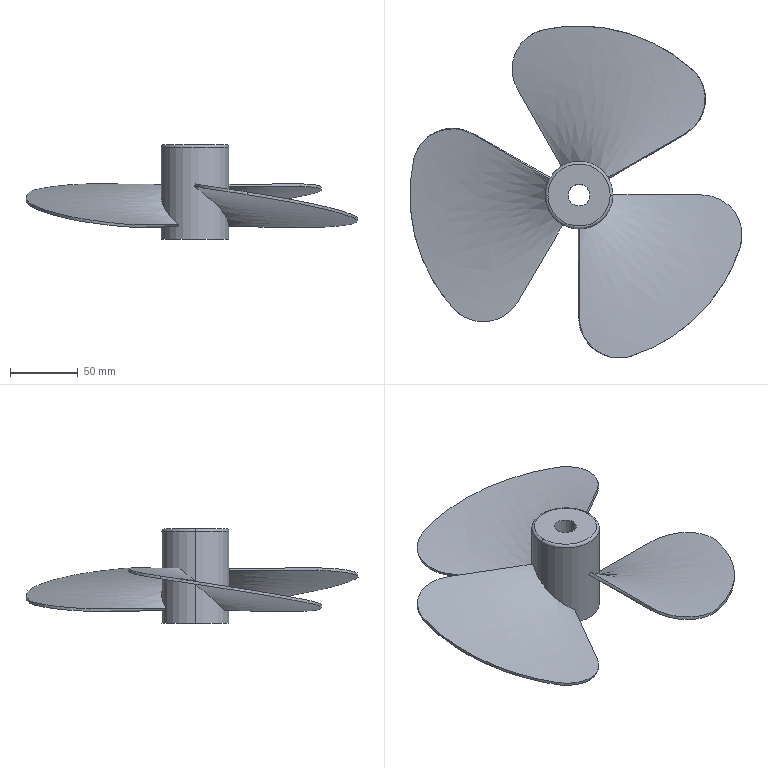Part | SolidWorks | features Fillet 2, CirPattern 1, Extrusion 1, Helix 1, RefAxis 1, SweepRefSurface 1, Thicken 1 | 4 solids | 32 faces | box 245.378 x 245.378 x 70 mm | volume 192980 mm3 | spline 24 | cylinder 4 | torus 2 | plane 2 | commonest cylinder face diameters 16 x2 50 x2